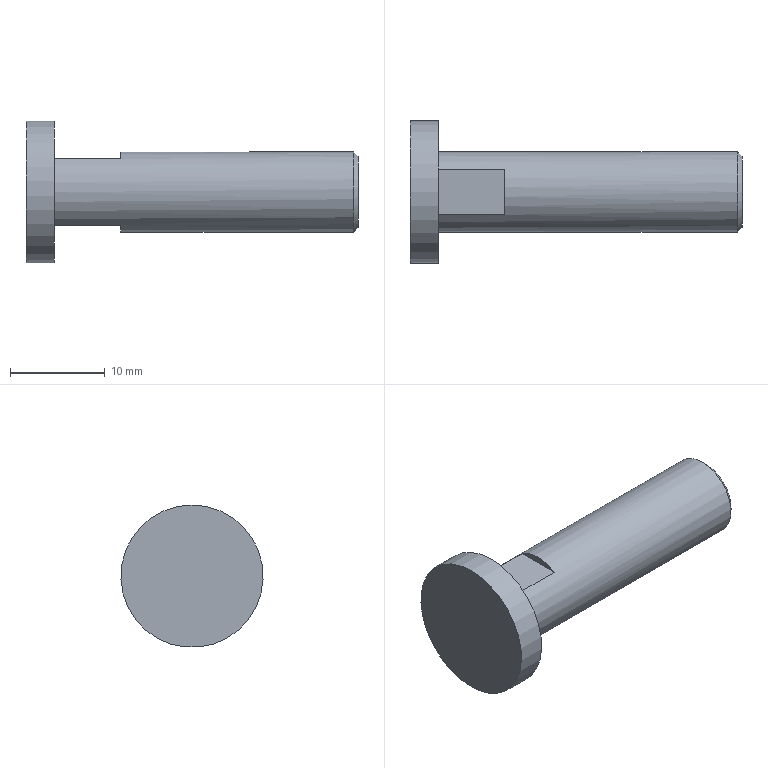Part | NX | features BREP 1 | 1 solid | 12 faces | box 35 x 15 x 15 mm | volume 2131 mm3 | plane 7 | cylinder 3 | cone 2 | commonest cylinder face diameters 4.2 x1 8.5 x1 15 x1
STEP:
#1=CARTESIAN_POINT('',(15.5,0.,4.25));
#2=VERTEX_POINT('',#1);
#3=CARTESIAN_POINT('',(15.5,0.,0.));
#4=DIRECTION('',(-1.,0.,0.));
#5=DIRECTION('',(0.,0.,1.));
#6=AXIS2_PLACEMENT_3D('',#3,#4,#5);
#7=CIRCLE('',#6,4.25);
#8=EDGE_CURVE('',#2,#2,#7,.T.);
#9=ORIENTED_EDGE('',*,*,#8,.T.);
#10=EDGE_LOOP('',(#9));
#11=FACE_BOUND('',#10,.T.);
#12=CARTESIAN_POINT('',(-9.,2.411,3.5));
#13=VERTEX_POINT('',#12);
#14=CARTESIAN_POINT('',(-16.,2.411,3.5));
#15=VERTEX_POINT('',#14);
#16=CARTESIAN_POINT('',(-16.,2.411,3.5));
#17=DIRECTION('',(-1.,0.,0.));
#18=VECTOR('',#17,1000.);
#19=LINE('',#16,#18);
#20=EDGE_CURVE('',#13,#15,#19,.T.);
#21=ORIENTED_EDGE('',*,*,#20,.F.);
#22=CARTESIAN_POINT('',(-9.,-2.411,3.5));
#23=VERTEX_POINT('',#22);
#24=CARTESIAN_POINT('',(-9.,0.,0.));
#25=DIRECTION('',(1.,0.,0.));
#26=DIRECTION('',(0.,0.,-1.));
#27=AXIS2_PLACEMENT_3D('',#24,#25,#26);
#28=CIRCLE('',#27,4.25);
#29=EDGE_CURVE('',#13,#23,#28,.T.);
#30=ORIENTED_EDGE('',*,*,#29,.T.);
#31=CARTESIAN_POINT('',(-16.,-2.411,3.5));
#32=VERTEX_POINT('',#31);
#33=CARTESIAN_POINT('',(-16.,-2.411,3.5));
#34=DIRECTION('',(1.,0.,0.));
#35=VECTOR('',#34,1000.);
#36=LINE('',#33,#35);
#37=EDGE_CURVE('',#32,#23,#36,.T.);
#38=ORIENTED_EDGE('',*,*,#37,.F.);
#39=CARTESIAN_POINT('',(-16.,-2.411,-3.5));
#40=VERTEX_POINT('',#39);
#41=CARTESIAN_POINT('',(-16.,0.,0.));
#42=DIRECTION('',(-1.,0.,0.));
#43=DIRECTION('',(0.,0.,1.));
#44=AXIS2_PLACEMENT_3D('',#41,#42,#43);
#45=CIRCLE('',#44,4.25);
#46=EDGE_CURVE('',#40,#32,#45,.T.);
#47=ORIENTED_EDGE('',*,*,#46,.F.);
#48=CARTESIAN_POINT('',(-9.,-2.411,-3.5));
#49=VERTEX_POINT('',#48);
#50=CARTESIAN_POINT('',(-16.,-2.411,-3.5));
#51=DIRECTION('',(-1.,0.,0.));
#52=VECTOR('',#51,1000.);
#53=LINE('',#50,#52);
#54=EDGE_CURVE('',#49,#40,#53,.T.);
#55=ORIENTED_EDGE('',*,*,#54,.F.);
#56=CARTESIAN_POINT('',(-9.,2.411,-3.5));
#57=VERTEX_POINT('',#56);
#58=CARTESIAN_POINT('',(-9.,0.,0.));
#59=DIRECTION('',(-1.,0.,0.));
#60=DIRECTION('',(0.,0.,1.));
#61=AXIS2_PLACEMENT_3D('',#58,#59,#60);
#62=CIRCLE('',#61,4.25);
#63=EDGE_CURVE('',#57,#49,#62,.T.);
#64=ORIENTED_EDGE('',*,*,#63,.F.);
#65=CARTESIAN_POINT('',(-16.,2.411,-3.5));
#66=VERTEX_POINT('',#65);
#67=CARTESIAN_POINT('',(-16.,2.411,-3.5));
#68=DIRECTION('',(1.,0.,0.));
#69=VECTOR('',#68,1000.);
#70=LINE('',#67,#69);
#71=EDGE_CURVE('',#66,#57,#70,.T.);
#72=ORIENTED_EDGE('',*,*,#71,.F.);
#73=CARTESIAN_POINT('',(-16.,0.,0.));
#74=DIRECTION('',(-1.,0.,0.));
#75=DIRECTION('',(0.,0.,1.));
#76=AXIS2_PLACEMENT_3D('',#73,#74,#75);
#77=CIRCLE('',#76,4.25);
#78=EDGE_CURVE('',#15,#66,#77,.T.);
#79=ORIENTED_EDGE('',*,*,#78,.F.);
#80=EDGE_LOOP('',(#21,#30,#38,#47,#55,#64,#72,#79));
#81=FACE_BOUND('',#80,.T.);
#82=CARTESIAN_POINT('',(-16.,0.,0.));
#83=DIRECTION('',(-1.,0.,0.));
#84=DIRECTION('',(0.,0.,-1.));
#85=AXIS2_PLACEMENT_3D('',#82,#83,#84);
#86=CYLINDRICAL_SURFACE('',#85,4.25);
#87=ADVANCED_FACE('',(#11,#81),#86,.T.);
#88=CARTESIAN_POINT('',(16.,0.,3.75));
#89=VERTEX_POINT('',#88);
#90=CARTESIAN_POINT('',(16.,0.,0.));
#91=DIRECTION('',(1.,0.,0.));
#92=DIRECTION('',(0.,0.,1.));
#93=AXIS2_PLACEMENT_3D('',#90,#91,#92);
#94=CIRCLE('',#93,3.75);
#95=EDGE_CURVE('',#89,#89,#94,.T.);
#96=ORIENTED_EDGE('',*,*,#95,.T.);
#97=EDGE_LOOP('',(#96));
#98=FACE_BOUND('',#97,.T.);
#99=CARTESIAN_POINT('',(16.,0.,-2.1));
#100=VERTEX_POINT('',#99);
#101=CARTESIAN_POINT('',(16.,0.,0.));
#102=DIRECTION('',(1.,0.,0.));
#103=DIRECTION('',(0.,0.,-1.));
#104=AXIS2_PLACEMENT_3D('',#101,#102,#103);
#105=CIRCLE('',#104,2.1);
#106=EDGE_CURVE('',#100,#100,#105,.T.);
#107=ORIENTED_EDGE('',*,*,#106,.F.);
#108=EDGE_LOOP('',(#107));
#109=FACE_BOUND('',#108,.T.);
#110=CARTESIAN_POINT('',(16.,0.,0.));
#111=DIRECTION('',(-1.,0.,0.));
#112=DIRECTION('',(0.,0.,-1.));
#113=AXIS2_PLACEMENT_3D('',#110,#111,#112);
#114=PLANE('',#113);
#115=ADVANCED_FACE('',(#98,#109),#114,.F.);
#116=CARTESIAN_POINT('',(2.338,0.,0.));
#117=VERTEX_POINT('',#116);
#118=VERTEX_LOOP('',#117);
#119=FACE_BOUND('',#118,.T.);
#120=CARTESIAN_POINT('',(3.6,0.,-2.1));
#121=VERTEX_POINT('',#120);
#122=CARTESIAN_POINT('',(3.6,0.,0.));
#123=DIRECTION('',(1.,0.,0.));
#124=DIRECTION('',(0.,0.,-1.));
#125=AXIS2_PLACEMENT_3D('',#122,#123,#124);
#126=CIRCLE('',#125,2.1);
#127=EDGE_CURVE('',#121,#121,#126,.T.);
#128=ORIENTED_EDGE('',*,*,#127,.T.);
#129=EDGE_LOOP('',(#128));
#130=FACE_BOUND('',#129,.T.);
#131=CARTESIAN_POINT('',(3.6,0.,0.));
#132=DIRECTION('',(1.,0.,0.));
#133=DIRECTION('',(0.,0.,1.));
#134=AXIS2_PLACEMENT_3D('',#131,#132,#133);
#135=CONICAL_SURFACE('',#134,2.1,1.03);
#136=ADVANCED_FACE('',(#119,#130),#135,.F.);
#137=ORIENTED_EDGE('',*,*,#127,.F.);
#138=EDGE_LOOP('',(#137));
#139=FACE_BOUND('',#138,.T.);
#140=ORIENTED_EDGE('',*,*,#106,.T.);
#141=EDGE_LOOP('',(#140));
#142=FACE_BOUND('',#141,.T.);
#143=CARTESIAN_POINT('',(16.,0.,0.));
#144=DIRECTION('',(1.,0.,0.));
#145=DIRECTION('',(0.,0.,1.));
#146=AXIS2_PLACEMENT_3D('',#143,#144,#145);
#147=CYLINDRICAL_SURFACE('',#146,2.1);
#148=ADVANCED_FACE('',(#139,#142),#147,.F.);
#149=CARTESIAN_POINT('',(-19.,0.,7.5));
#150=VERTEX_POINT('',#149);
#151=CARTESIAN_POINT('',(-19.,0.,0.));
#152=DIRECTION('',(-1.,0.,0.));
#153=DIRECTION('',(0.,0.,1.));
#154=AXIS2_PLACEMENT_3D('',#151,#152,#153);
#155=CIRCLE('',#154,7.5);
#156=EDGE_CURVE('',#150,#150,#155,.T.);
#157=ORIENTED_EDGE('',*,*,#156,.F.);
#158=EDGE_LOOP('',(#157));
#159=FACE_BOUND('',#158,.T.);
#160=CARTESIAN_POINT('',(-16.,0.,7.5));
#161=VERTEX_POINT('',#160);
#162=CARTESIAN_POINT('',(-16.,0.,0.));
#163=DIRECTION('',(-1.,0.,0.));
#164=DIRECTION('',(0.,0.,1.));
#165=AXIS2_PLACEMENT_3D('',#162,#163,#164);
#166=CIRCLE('',#165,7.5);
#167=EDGE_CURVE('',#161,#161,#166,.T.);
#168=ORIENTED_EDGE('',*,*,#167,.T.);
#169=EDGE_LOOP('',(#168));
#170=FACE_BOUND('',#169,.T.);
#171=CARTESIAN_POINT('',(-19.,0.,0.));
#172=DIRECTION('',(1.,0.,0.));
#173=DIRECTION('',(0.,0.,1.));
#174=AXIS2_PLACEMENT_3D('',#171,#172,#173);
#175=CYLINDRICAL_SURFACE('',#174,7.5);
#176=ADVANCED_FACE('',(#159,#170),#175,.T.);
#177=ORIENTED_EDGE('',*,*,#156,.T.);
#178=EDGE_LOOP('',(#177));
#179=FACE_BOUND('',#178,.T.);
#180=CARTESIAN_POINT('',(-19.,0.,0.));
#181=DIRECTION('',(-1.,0.,0.));
#182=DIRECTION('',(0.,0.,-1.));
#183=AXIS2_PLACEMENT_3D('',#180,#181,#182);
#184=PLANE('',#183);
#185=ADVANCED_FACE('',(#179),#184,.T.);
#186=ORIENTED_EDGE('',*,*,#46,.T.);
#187=CARTESIAN_POINT('',(-16.,5.351,3.5));
#188=DIRECTION('',(0.,1.,0.));
#189=VECTOR('',#188,1000.);
#190=LINE('',#187,#189);
#191=EDGE_CURVE('',#32,#15,#190,.T.);
#192=ORIENTED_EDGE('',*,*,#191,.T.);
#193=ORIENTED_EDGE('',*,*,#78,.T.);
#194=CARTESIAN_POINT('',(-16.,3.784,-3.5));
#195=DIRECTION('',(0.,-1.,0.));
#196=VECTOR('',#195,1000.);
#197=LINE('',#194,#196);
#198=EDGE_CURVE('',#66,#40,#197,.T.);
#199=ORIENTED_EDGE('',*,*,#198,.T.);
#200=EDGE_LOOP('',(#186,#192,#193,#199));
#201=FACE_BOUND('',#200,.T.);
#202=ORIENTED_EDGE('',*,*,#167,.F.);
#203=EDGE_LOOP('',(#202));
#204=FACE_BOUND('',#203,.T.);
#205=CARTESIAN_POINT('',(-16.,0.,0.));
#206=DIRECTION('',(-1.,0.,0.));
#207=DIRECTION('',(0.,0.,-1.));
#208=AXIS2_PLACEMENT_3D('',#205,#206,#207);
#209=PLANE('',#208);
#210=ADVANCED_FACE('',(#201,#204),#209,.F.);
#211=ORIENTED_EDGE('',*,*,#95,.F.);
#212=EDGE_LOOP('',(#211));
#213=FACE_BOUND('',#212,.T.);
#214=ORIENTED_EDGE('',*,*,#8,.F.);
#215=EDGE_LOOP('',(#214));
#216=FACE_BOUND('',#215,.T.);
#217=CARTESIAN_POINT('',(15.5,0.,0.));
#218=DIRECTION('',(-1.,0.,0.));
#219=DIRECTION('',(0.,0.,-1.));
#220=AXIS2_PLACEMENT_3D('',#217,#218,#219);
#221=CONICAL_SURFACE('',#220,4.25,0.7854);
#222=ADVANCED_FACE('',(#213,#216),#221,.T.);
#223=ORIENTED_EDGE('',*,*,#63,.T.);
#224=CARTESIAN_POINT('',(-9.,3.784,-3.5));
#225=DIRECTION('',(0.,-1.,0.));
#226=VECTOR('',#225,1000.);
#227=LINE('',#224,#226);
#228=EDGE_CURVE('',#57,#49,#227,.T.);
#229=ORIENTED_EDGE('',*,*,#228,.F.);
#230=EDGE_LOOP('',(#223,#229));
#231=FACE_BOUND('',#230,.T.);
#232=CARTESIAN_POINT('',(-9.,0.,0.));
#233=DIRECTION('',(-1.,0.,0.));
#234=DIRECTION('',(0.,0.,-1.));
#235=AXIS2_PLACEMENT_3D('',#232,#233,#234);
#236=PLANE('',#235);
#237=ADVANCED_FACE('',(#231),#236,.T.);
#238=ORIENTED_EDGE('',*,*,#54,.T.);
#239=ORIENTED_EDGE('',*,*,#198,.F.);
#240=ORIENTED_EDGE('',*,*,#71,.T.);
#241=ORIENTED_EDGE('',*,*,#228,.T.);
#242=EDGE_LOOP('',(#238,#239,#240,#241));
#243=FACE_BOUND('',#242,.T.);
#244=CARTESIAN_POINT('',(-9.,3.784,-3.5));
#245=DIRECTION('',(0.,0.,-1.));
#246=DIRECTION('',(0.,-1.,0.));
#247=AXIS2_PLACEMENT_3D('',#244,#245,#246);
#248=PLANE('',#247);
#249=ADVANCED_FACE('',(#243),#248,.T.);
#250=CARTESIAN_POINT('',(-9.,5.351,3.5));
#251=DIRECTION('',(0.,1.,0.));
#252=VECTOR('',#251,1000.);
#253=LINE('',#250,#252);
#254=EDGE_CURVE('',#23,#13,#253,.T.);
#255=ORIENTED_EDGE('',*,*,#254,.F.);
#256=ORIENTED_EDGE('',*,*,#29,.F.);
#257=EDGE_LOOP('',(#255,#256));
#258=FACE_BOUND('',#257,.T.);
#259=CARTESIAN_POINT('',(-9.,0.,0.));
#260=DIRECTION('',(1.,0.,0.));
#261=DIRECTION('',(0.,0.,1.));
#262=AXIS2_PLACEMENT_3D('',#259,#260,#261);
#263=PLANE('',#262);
#264=ADVANCED_FACE('',(#258),#263,.F.);
#265=ORIENTED_EDGE('',*,*,#20,.T.);
#266=ORIENTED_EDGE('',*,*,#191,.F.);
#267=ORIENTED_EDGE('',*,*,#37,.T.);
#268=ORIENTED_EDGE('',*,*,#254,.T.);
#269=EDGE_LOOP('',(#265,#266,#267,#268));
#270=FACE_BOUND('',#269,.T.);
#271=CARTESIAN_POINT('',(-9.,5.351,3.5));
#272=DIRECTION('',(0.,0.,1.));
#273=DIRECTION('',(0.,1.,0.));
#274=AXIS2_PLACEMENT_3D('',#271,#272,#273);
#275=PLANE('',#274);
#276=ADVANCED_FACE('',(#270),#275,.T.);
#277=CLOSED_SHELL('',(#87,#115,#136,#148,#176,#185,#210,#222,#237,#249,#264,#276));
#278=MANIFOLD_SOLID_BREP('',#277);
#279=(LENGTH_UNIT()NAMED_UNIT(*)SI_UNIT(.MILLI.,.METRE.));
#280=UNCERTAINTY_MEASURE_WITH_UNIT(LENGTH_MEASURE(0.00001),#279,'','');
#281=(NAMED_UNIT(*)PLANE_ANGLE_UNIT()SI_UNIT($,.RADIAN.));
#282=(NAMED_UNIT(*)SI_UNIT($,.STERADIAN.)SOLID_ANGLE_UNIT());
#283=(GEOMETRIC_REPRESENTATION_CONTEXT(3)GLOBAL_UNCERTAINTY_ASSIGNED_CONTEXT((#280))GLOBAL_UNIT_ASSIGNED_CONTEXT((#279,#281,#282))REPRESENTATION_CONTEXT('',''));
#284=ADVANCED_BREP_SHAPE_REPRESENTATION('',(#278),#283);